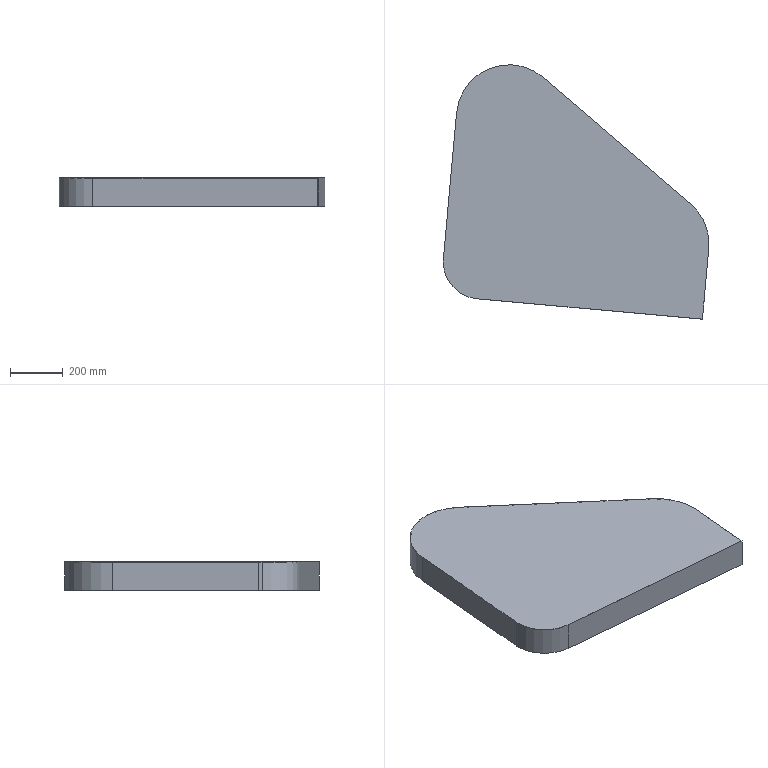Part | SolidWorks | features Extrusion 1, Shell 1 | 1 solid | 19 faces | box 1010 x 967.019 x 110 mm | volume 3119337 mm3 | plane 11 | cylinder 8 | commonest cylinder face diameters 274 x2 280 x2 394 x2 400 x2
STEP:
#1=CARTESIAN_POINT('',(-246.443,-537.657,107.));
#2=VERTEX_POINT('',#1);
#3=CARTESIAN_POINT('',(-247.,-550.,107.));
#4=VERTEX_POINT('',#3);
#5=CARTESIAN_POINT('',(-110.,-550.,107.));
#6=DIRECTION('',(0.,0.,1.));
#7=DIRECTION('',(1.,0.,0.));
#8=AXIS2_PLACEMENT_3D('',#5,#6,#7);
#9=CIRCLE('',#8,137.);
#10=EDGE_CURVE('',#2,#4,#9,.T.);
#11=ORIENTED_EDGE('',*,*,#10,.T.);
#12=CARTESIAN_POINT('',(-247.,-550.,0.));
#13=VERTEX_POINT('',#12);
#14=CARTESIAN_POINT('',(-247.,-550.,110.));
#15=DIRECTION('',(0.,0.,-1.));
#16=VECTOR('',#15,1000.);
#17=LINE('',#14,#16);
#18=EDGE_CURVE('',#4,#13,#17,.T.);
#19=ORIENTED_EDGE('',*,*,#18,.T.);
#20=CARTESIAN_POINT('',(-246.443,-537.657,0.));
#21=VERTEX_POINT('',#20);
#22=CARTESIAN_POINT('',(-110.,-550.,0.));
#23=DIRECTION('',(0.,0.,1.));
#24=DIRECTION('',(1.,0.,0.));
#25=AXIS2_PLACEMENT_3D('',#22,#23,#24);
#26=CIRCLE('',#25,137.);
#27=EDGE_CURVE('',#21,#13,#26,.T.);
#28=ORIENTED_EDGE('',*,*,#27,.F.);
#29=CARTESIAN_POINT('',(-246.443,-537.657,110.));
#30=DIRECTION('',(0.,0.,-1.));
#31=VECTOR('',#30,1000.);
#32=LINE('',#29,#31);
#33=EDGE_CURVE('',#2,#21,#32,.T.);
#34=ORIENTED_EDGE('',*,*,#33,.F.);
#35=EDGE_LOOP('',(#11,#19,#28,#34));
#36=FACE_OUTER_BOUND('',#35,.T.);
#37=CARTESIAN_POINT('',(-110.,-550.,110.));
#38=DIRECTION('',(0.,0.,-1.));
#39=DIRECTION('',(-1.,0.,0.));
#40=AXIS2_PLACEMENT_3D('',#37,#38,#39);
#41=CYLINDRICAL_SURFACE('',#40,137.);
#42=ADVANCED_FACE('',(#36),#41,.F.);
#43=CARTESIAN_POINT('',(-250.,-550.,110.));
#44=VERTEX_POINT('',#43);
#45=CARTESIAN_POINT('',(-122.613,-689.431,110.));
#46=VERTEX_POINT('',#45);
#47=CARTESIAN_POINT('',(-110.,-550.,110.));
#48=DIRECTION('',(0.,0.,1.));
#49=DIRECTION('',(1.,0.,0.));
#50=AXIS2_PLACEMENT_3D('',#47,#48,#49);
#51=CIRCLE('',#50,140.);
#52=EDGE_CURVE('',#44,#46,#51,.T.);
#53=ORIENTED_EDGE('',*,*,#52,.F.);
#54=CARTESIAN_POINT('',(-250.,-550.,0.));
#55=VERTEX_POINT('',#54);
#56=CARTESIAN_POINT('',(-250.,-550.,110.));
#57=DIRECTION('',(0.,0.,-1.));
#58=VECTOR('',#57,1000.);
#59=LINE('',#56,#58);
#60=EDGE_CURVE('',#44,#55,#59,.T.);
#61=ORIENTED_EDGE('',*,*,#60,.T.);
#62=CARTESIAN_POINT('',(-122.613,-689.431,0.));
#63=VERTEX_POINT('',#62);
#64=CARTESIAN_POINT('',(-110.,-550.,0.));
#65=DIRECTION('',(0.,0.,1.));
#66=DIRECTION('',(1.,0.,0.));
#67=AXIS2_PLACEMENT_3D('',#64,#65,#66);
#68=CIRCLE('',#67,140.);
#69=EDGE_CURVE('',#55,#63,#68,.T.);
#70=ORIENTED_EDGE('',*,*,#69,.T.);
#71=CARTESIAN_POINT('',(-122.613,-689.431,110.));
#72=DIRECTION('',(0.,0.,-1.));
#73=VECTOR('',#72,1000.);
#74=LINE('',#71,#73);
#75=EDGE_CURVE('',#46,#63,#74,.T.);
#76=ORIENTED_EDGE('',*,*,#75,.F.);
#77=EDGE_LOOP('',(#53,#61,#70,#76));
#78=FACE_OUTER_BOUND('',#77,.T.);
#79=CARTESIAN_POINT('',(-110.,-550.,110.));
#80=DIRECTION('',(0.,0.,-1.));
#81=DIRECTION('',(-1.,0.,0.));
#82=AXIS2_PLACEMENT_3D('',#79,#80,#81);
#83=CYLINDRICAL_SURFACE('',#82,140.);
#84=ADVANCED_FACE('',(#78),#83,.T.);
#85=CARTESIAN_POINT('',(130.202,151.814,0.));
#86=VERTEX_POINT('',#85);
#87=CARTESIAN_POINT('',(-199.187,18.019,0.));
#88=VERTEX_POINT('',#87);
#89=CARTESIAN_POINT('',(0.,0.,0.));
#90=DIRECTION('',(0.,0.,1.));
#91=DIRECTION('',(1.,0.,0.));
#92=AXIS2_PLACEMENT_3D('',#89,#90,#91);
#93=CIRCLE('',#92,200.);
#94=EDGE_CURVE('',#86,#88,#93,.T.);
#95=ORIENTED_EDGE('',*,*,#94,.T.);
#96=CARTESIAN_POINT('',(-199.187,18.019,110.));
#97=VERTEX_POINT('',#96);
#98=CARTESIAN_POINT('',(-199.187,18.019,110.));
#99=DIRECTION('',(0.,0.,-1.));
#100=VECTOR('',#99,1000.);
#101=LINE('',#98,#100);
#102=EDGE_CURVE('',#97,#88,#101,.T.);
#103=ORIENTED_EDGE('',*,*,#102,.F.);
#104=CARTESIAN_POINT('',(130.202,151.814,110.));
#105=VERTEX_POINT('',#104);
#106=CARTESIAN_POINT('',(0.,0.,110.));
#107=DIRECTION('',(0.,0.,1.));
#108=DIRECTION('',(1.,0.,0.));
#109=AXIS2_PLACEMENT_3D('',#106,#107,#108);
#110=CIRCLE('',#109,200.);
#111=EDGE_CURVE('',#105,#97,#110,.T.);
#112=ORIENTED_EDGE('',*,*,#111,.F.);
#113=CARTESIAN_POINT('',(130.202,151.814,110.));
#114=DIRECTION('',(0.,0.,-1.));
#115=VECTOR('',#114,1000.);
#116=LINE('',#113,#115);
#117=EDGE_CURVE('',#105,#86,#116,.T.);
#118=ORIENTED_EDGE('',*,*,#117,.T.);
#119=EDGE_LOOP('',(#95,#103,#112,#118));
#120=FACE_OUTER_BOUND('',#119,.T.);
#121=CARTESIAN_POINT('',(0.,0.,110.));
#122=DIRECTION('',(0.,0.,-1.));
#123=DIRECTION('',(-1.,0.,0.));
#124=AXIS2_PLACEMENT_3D('',#121,#122,#123);
#125=CYLINDRICAL_SURFACE('',#124,200.);
#126=ADVANCED_FACE('',(#120),#125,.T.);
#127=CARTESIAN_POINT('',(-249.431,-537.387,0.));
#128=VERTEX_POINT('',#127);
#129=CARTESIAN_POINT('',(-199.187,18.019,0.));
#130=DIRECTION('',(-0.0901,-0.9959,0.));
#131=VECTOR('',#130,1000.);
#132=LINE('',#129,#131);
#133=EDGE_CURVE('',#88,#128,#132,.T.);
#134=ORIENTED_EDGE('',*,*,#133,.T.);
#135=CARTESIAN_POINT('',(-249.431,-537.387,110.));
#136=VERTEX_POINT('',#135);
#137=CARTESIAN_POINT('',(-249.431,-537.387,110.));
#138=DIRECTION('',(0.,0.,-1.));
#139=VECTOR('',#138,1000.);
#140=LINE('',#137,#139);
#141=EDGE_CURVE('',#136,#128,#140,.T.);
#142=ORIENTED_EDGE('',*,*,#141,.F.);
#143=CARTESIAN_POINT('',(-199.187,18.019,110.));
#144=DIRECTION('',(-0.0901,-0.9959,0.));
#145=VECTOR('',#144,1000.);
#146=LINE('',#143,#145);
#147=EDGE_CURVE('',#97,#136,#146,.T.);
#148=ORIENTED_EDGE('',*,*,#147,.F.);
#149=ORIENTED_EDGE('',*,*,#102,.T.);
#150=EDGE_LOOP('',(#134,#142,#148,#149));
#151=FACE_OUTER_BOUND('',#150,.T.);
#152=CARTESIAN_POINT('',(-199.187,18.019,110.));
#153=DIRECTION('',(0.9959,-0.0901,0.));
#154=DIRECTION('',(0.0901,0.9959,0.));
#155=AXIS2_PLACEMENT_3D('',#152,#153,#154);
#156=PLANE('',#155);
#157=ADVANCED_FACE('',(#151),#156,.F.);
#158=ORIENTED_EDGE('',*,*,#60,.F.);
#159=CARTESIAN_POINT('',(-110.,-550.,110.));
#160=DIRECTION('',(0.,0.,1.));
#161=DIRECTION('',(1.,0.,0.));
#162=AXIS2_PLACEMENT_3D('',#159,#160,#161);
#163=CIRCLE('',#162,140.);
#164=EDGE_CURVE('',#136,#44,#163,.T.);
#165=ORIENTED_EDGE('',*,*,#164,.F.);
#166=ORIENTED_EDGE('',*,*,#141,.T.);
#167=CARTESIAN_POINT('',(-110.,-550.,0.));
#168=DIRECTION('',(0.,0.,1.));
#169=DIRECTION('',(1.,0.,0.));
#170=AXIS2_PLACEMENT_3D('',#167,#168,#169);
#171=CIRCLE('',#170,140.);
#172=EDGE_CURVE('',#128,#55,#171,.T.);
#173=ORIENTED_EDGE('',*,*,#172,.T.);
#174=EDGE_LOOP('',(#158,#165,#166,#173));
#175=FACE_OUTER_BOUND('',#174,.T.);
#176=CARTESIAN_POINT('',(-110.,-550.,110.));
#177=DIRECTION('',(0.,0.,-1.));
#178=DIRECTION('',(-1.,0.,0.));
#179=AXIS2_PLACEMENT_3D('',#176,#177,#178);
#180=CYLINDRICAL_SURFACE('',#179,140.);
#181=ADVANCED_FACE('',(#175),#180,.T.);
#182=CARTESIAN_POINT('',(735.06,-767.019,0.));
#183=VERTEX_POINT('',#182);
#184=CARTESIAN_POINT('',(-122.613,-689.431,0.));
#185=DIRECTION('',(0.9959,-0.0901,0.));
#186=VECTOR('',#185,1000.);
#187=LINE('',#184,#186);
#188=EDGE_CURVE('',#63,#183,#187,.T.);
#189=ORIENTED_EDGE('',*,*,#188,.T.);
#190=CARTESIAN_POINT('',(735.06,-767.019,110.));
#191=VERTEX_POINT('',#190);
#192=CARTESIAN_POINT('',(735.06,-767.019,110.));
#193=DIRECTION('',(0.,0.,-1.));
#194=VECTOR('',#193,1000.);
#195=LINE('',#192,#194);
#196=EDGE_CURVE('',#191,#183,#195,.T.);
#197=ORIENTED_EDGE('',*,*,#196,.F.);
#198=CARTESIAN_POINT('',(-122.613,-689.431,110.));
#199=DIRECTION('',(0.9959,-0.0901,0.));
#200=VECTOR('',#199,1000.);
#201=LINE('',#198,#200);
#202=EDGE_CURVE('',#46,#191,#201,.T.);
#203=ORIENTED_EDGE('',*,*,#202,.F.);
#204=ORIENTED_EDGE('',*,*,#75,.T.);
#205=EDGE_LOOP('',(#189,#197,#203,#204));
#206=FACE_OUTER_BOUND('',#205,.T.);
#207=CARTESIAN_POINT('',(-122.613,-689.431,110.));
#208=DIRECTION('',(0.0901,0.9959,0.));
#209=DIRECTION('',(-0.9959,0.0901,0.));
#210=AXIS2_PLACEMENT_3D('',#207,#208,#209);
#211=PLANE('',#210);
#212=ADVANCED_FACE('',(#206),#211,.F.);
#213=CARTESIAN_POINT('',(759.356,-498.442,0.));
#214=VERTEX_POINT('',#213);
#215=CARTESIAN_POINT('',(759.356,-498.442,0.));
#216=DIRECTION('',(0.0901,0.9959,0.));
#217=VECTOR('',#216,1000.);
#218=LINE('',#215,#217);
#219=EDGE_CURVE('',#183,#214,#218,.T.);
#220=ORIENTED_EDGE('',*,*,#219,.T.);
#221=CARTESIAN_POINT('',(759.356,-498.442,110.));
#222=VERTEX_POINT('',#221);
#223=CARTESIAN_POINT('',(759.356,-498.442,110.));
#224=DIRECTION('',(0.,0.,-1.));
#225=VECTOR('',#224,1000.);
#226=LINE('',#223,#225);
#227=EDGE_CURVE('',#222,#214,#226,.T.);
#228=ORIENTED_EDGE('',*,*,#227,.F.);
#229=CARTESIAN_POINT('',(759.356,-498.442,110.));
#230=DIRECTION('',(0.0901,0.9959,0.));
#231=VECTOR('',#230,1000.);
#232=LINE('',#229,#231);
#233=EDGE_CURVE('',#191,#222,#232,.T.);
#234=ORIENTED_EDGE('',*,*,#233,.F.);
#235=ORIENTED_EDGE('',*,*,#196,.T.);
#236=EDGE_LOOP('',(#220,#228,#234,#235));
#237=FACE_OUTER_BOUND('',#236,.T.);
#238=CARTESIAN_POINT('',(759.356,-498.442,110.));
#239=DIRECTION('',(-0.9959,0.0901,0.));
#240=DIRECTION('',(-0.0901,-0.9959,0.));
#241=AXIS2_PLACEMENT_3D('',#238,#239,#240);
#242=PLANE('',#241);
#243=ADVANCED_FACE('',(#237),#242,.F.);
#244=CARTESIAN_POINT('',(690.371,-328.609,0.));
#245=VERTEX_POINT('',#244);
#246=CARTESIAN_POINT('',(560.17,-480.423,0.));
#247=DIRECTION('',(0.,0.,1.));
#248=DIRECTION('',(1.,0.,0.));
#249=AXIS2_PLACEMENT_3D('',#246,#247,#248);
#250=CIRCLE('',#249,200.);
#251=EDGE_CURVE('',#214,#245,#250,.T.);
#252=ORIENTED_EDGE('',*,*,#251,.T.);
#253=CARTESIAN_POINT('',(690.371,-328.609,110.));
#254=VERTEX_POINT('',#253);
#255=CARTESIAN_POINT('',(690.371,-328.609,110.));
#256=DIRECTION('',(0.,0.,-1.));
#257=VECTOR('',#256,1000.);
#258=LINE('',#255,#257);
#259=EDGE_CURVE('',#254,#245,#258,.T.);
#260=ORIENTED_EDGE('',*,*,#259,.F.);
#261=CARTESIAN_POINT('',(560.17,-480.423,110.));
#262=DIRECTION('',(0.,0.,1.));
#263=DIRECTION('',(1.,0.,0.));
#264=AXIS2_PLACEMENT_3D('',#261,#262,#263);
#265=CIRCLE('',#264,200.);
#266=EDGE_CURVE('',#222,#254,#265,.T.);
#267=ORIENTED_EDGE('',*,*,#266,.F.);
#268=ORIENTED_EDGE('',*,*,#227,.T.);
#269=EDGE_LOOP('',(#252,#260,#267,#268));
#270=FACE_OUTER_BOUND('',#269,.T.);
#271=CARTESIAN_POINT('',(560.17,-480.423,110.));
#272=DIRECTION('',(0.,0.,-1.));
#273=DIRECTION('',(-1.,0.,0.));
#274=AXIS2_PLACEMENT_3D('',#271,#272,#273);
#275=CYLINDRICAL_SURFACE('',#274,200.);
#276=ADVANCED_FACE('',(#270),#275,.T.);
#277=CARTESIAN_POINT('',(130.202,151.814,0.));
#278=DIRECTION('',(-0.7591,0.651,0.));
#279=VECTOR('',#278,1000.);
#280=LINE('',#277,#279);
#281=EDGE_CURVE('',#245,#86,#280,.T.);
#282=ORIENTED_EDGE('',*,*,#281,.T.);
#283=ORIENTED_EDGE('',*,*,#117,.F.);
#284=CARTESIAN_POINT('',(130.202,151.814,110.));
#285=DIRECTION('',(-0.7591,0.651,0.));
#286=VECTOR('',#285,1000.);
#287=LINE('',#284,#286);
#288=EDGE_CURVE('',#254,#105,#287,.T.);
#289=ORIENTED_EDGE('',*,*,#288,.F.);
#290=ORIENTED_EDGE('',*,*,#259,.T.);
#291=EDGE_LOOP('',(#282,#283,#289,#290));
#292=FACE_OUTER_BOUND('',#291,.T.);
#293=CARTESIAN_POINT('',(130.202,151.814,110.));
#294=DIRECTION('',(-0.651,-0.7591,0.));
#295=DIRECTION('',(0.7591,-0.651,0.));
#296=AXIS2_PLACEMENT_3D('',#293,#294,#295);
#297=PLANE('',#296);
#298=ADVANCED_FACE('',(#292),#297,.F.);
#299=ORIENTED_EDGE('',*,*,#111,.T.);
#300=ORIENTED_EDGE('',*,*,#147,.T.);
#301=ORIENTED_EDGE('',*,*,#164,.T.);
#302=ORIENTED_EDGE('',*,*,#52,.T.);
#303=ORIENTED_EDGE('',*,*,#202,.T.);
#304=ORIENTED_EDGE('',*,*,#233,.T.);
#305=ORIENTED_EDGE('',*,*,#266,.T.);
#306=ORIENTED_EDGE('',*,*,#288,.T.);
#307=EDGE_LOOP('',(#299,#300,#301,#302,#303,#304,#305,#306));
#308=FACE_OUTER_BOUND('',#307,.T.);
#309=CARTESIAN_POINT('',(0.,0.,110.));
#310=DIRECTION('',(0.,0.,1.));
#311=DIRECTION('',(1.,0.,0.));
#312=AXIS2_PLACEMENT_3D('',#309,#310,#311);
#313=PLANE('',#312);
#314=ADVANCED_FACE('',(#308),#313,.T.);
#315=CARTESIAN_POINT('',(688.418,-330.886,0.));
#316=VERTEX_POINT('',#315);
#317=CARTESIAN_POINT('',(128.249,149.537,0.));
#318=VERTEX_POINT('',#317);
#319=CARTESIAN_POINT('',(128.249,149.537,0.));
#320=DIRECTION('',(-0.7591,0.651,0.));
#321=VECTOR('',#320,1000.);
#322=LINE('',#319,#321);
#323=EDGE_CURVE('',#316,#318,#322,.T.);
#324=ORIENTED_EDGE('',*,*,#323,.T.);
#325=CARTESIAN_POINT('',(-196.199,17.749,0.));
#326=VERTEX_POINT('',#325);
#327=CARTESIAN_POINT('',(0.,0.,0.));
#328=DIRECTION('',(0.,0.,1.));
#329=DIRECTION('',(1.,0.,0.));
#330=AXIS2_PLACEMENT_3D('',#327,#328,#329);
#331=CIRCLE('',#330,197.);
#332=EDGE_CURVE('',#318,#326,#331,.T.);
#333=ORIENTED_EDGE('',*,*,#332,.T.);
#334=CARTESIAN_POINT('',(-196.199,17.749,0.));
#335=DIRECTION('',(-0.0901,-0.9959,0.));
#336=VECTOR('',#335,1000.);
#337=LINE('',#334,#336);
#338=EDGE_CURVE('',#326,#21,#337,.T.);
#339=ORIENTED_EDGE('',*,*,#338,.T.);
#340=ORIENTED_EDGE('',*,*,#27,.T.);
#341=CARTESIAN_POINT('',(-122.343,-686.443,0.));
#342=VERTEX_POINT('',#341);
#343=CARTESIAN_POINT('',(-110.,-550.,0.));
#344=DIRECTION('',(0.,0.,1.));
#345=DIRECTION('',(1.,0.,0.));
#346=AXIS2_PLACEMENT_3D('',#343,#344,#345);
#347=CIRCLE('',#346,137.);
#348=EDGE_CURVE('',#13,#342,#347,.T.);
#349=ORIENTED_EDGE('',*,*,#348,.T.);
#350=CARTESIAN_POINT('',(732.342,-763.761,0.));
#351=VERTEX_POINT('',#350);
#352=CARTESIAN_POINT('',(-122.343,-686.443,0.));
#353=DIRECTION('',(0.9959,-0.0901,0.));
#354=VECTOR('',#353,1000.);
#355=LINE('',#352,#354);
#356=EDGE_CURVE('',#342,#351,#355,.T.);
#357=ORIENTED_EDGE('',*,*,#356,.T.);
#358=CARTESIAN_POINT('',(756.368,-498.172,0.));
#359=VERTEX_POINT('',#358);
#360=CARTESIAN_POINT('',(756.368,-498.172,0.));
#361=DIRECTION('',(0.0901,0.9959,0.));
#362=VECTOR('',#361,1000.);
#363=LINE('',#360,#362);
#364=EDGE_CURVE('',#351,#359,#363,.T.);
#365=ORIENTED_EDGE('',*,*,#364,.T.);
#366=CARTESIAN_POINT('',(560.17,-480.423,0.));
#367=DIRECTION('',(0.,0.,1.));
#368=DIRECTION('',(1.,0.,0.));
#369=AXIS2_PLACEMENT_3D('',#366,#367,#368);
#370=CIRCLE('',#369,197.);
#371=EDGE_CURVE('',#359,#316,#370,.T.);
#372=ORIENTED_EDGE('',*,*,#371,.T.);
#373=EDGE_LOOP('',(#324,#333,#339,#340,#349,#357,#365,#372));
#374=FACE_BOUND('',#373,.T.);
#375=ORIENTED_EDGE('',*,*,#94,.F.);
#376=ORIENTED_EDGE('',*,*,#281,.F.);
#377=ORIENTED_EDGE('',*,*,#251,.F.);
#378=ORIENTED_EDGE('',*,*,#219,.F.);
#379=ORIENTED_EDGE('',*,*,#188,.F.);
#380=ORIENTED_EDGE('',*,*,#69,.F.);
#381=ORIENTED_EDGE('',*,*,#172,.F.);
#382=ORIENTED_EDGE('',*,*,#133,.F.);
#383=EDGE_LOOP('',(#375,#376,#377,#378,#379,#380,#381,#382));
#384=FACE_OUTER_BOUND('',#383,.T.);
#385=CARTESIAN_POINT('',(0.,0.,0.));
#386=DIRECTION('',(0.,0.,1.));
#387=DIRECTION('',(1.,0.,0.));
#388=AXIS2_PLACEMENT_3D('',#385,#386,#387);
#389=PLANE('',#388);
#390=ADVANCED_FACE('',(#374,#384),#389,.F.);
#391=ORIENTED_EDGE('',*,*,#332,.F.);
#392=CARTESIAN_POINT('',(128.249,149.537,107.));
#393=VERTEX_POINT('',#392);
#394=CARTESIAN_POINT('',(128.249,149.537,110.));
#395=DIRECTION('',(0.,0.,-1.));
#396=VECTOR('',#395,1000.);
#397=LINE('',#394,#396);
#398=EDGE_CURVE('',#393,#318,#397,.T.);
#399=ORIENTED_EDGE('',*,*,#398,.F.);
#400=CARTESIAN_POINT('',(-196.199,17.749,107.));
#401=VERTEX_POINT('',#400);
#402=CARTESIAN_POINT('',(0.,0.,107.));
#403=DIRECTION('',(0.,0.,1.));
#404=DIRECTION('',(1.,0.,0.));
#405=AXIS2_PLACEMENT_3D('',#402,#403,#404);
#406=CIRCLE('',#405,197.);
#407=EDGE_CURVE('',#393,#401,#406,.T.);
#408=ORIENTED_EDGE('',*,*,#407,.T.);
#409=CARTESIAN_POINT('',(-196.199,17.749,110.));
#410=DIRECTION('',(0.,0.,-1.));
#411=VECTOR('',#410,1000.);
#412=LINE('',#409,#411);
#413=EDGE_CURVE('',#401,#326,#412,.T.);
#414=ORIENTED_EDGE('',*,*,#413,.T.);
#415=EDGE_LOOP('',(#391,#399,#408,#414));
#416=FACE_OUTER_BOUND('',#415,.T.);
#417=CARTESIAN_POINT('',(0.,0.,110.));
#418=DIRECTION('',(0.,0.,-1.));
#419=DIRECTION('',(-1.,0.,0.));
#420=AXIS2_PLACEMENT_3D('',#417,#418,#419);
#421=CYLINDRICAL_SURFACE('',#420,197.);
#422=ADVANCED_FACE('',(#416),#421,.F.);
#423=ORIENTED_EDGE('',*,*,#338,.F.);
#424=ORIENTED_EDGE('',*,*,#413,.F.);
#425=CARTESIAN_POINT('',(-196.199,17.749,107.));
#426=DIRECTION('',(-0.0901,-0.9959,0.));
#427=VECTOR('',#426,1000.);
#428=LINE('',#425,#427);
#429=EDGE_CURVE('',#401,#2,#428,.T.);
#430=ORIENTED_EDGE('',*,*,#429,.T.);
#431=ORIENTED_EDGE('',*,*,#33,.T.);
#432=EDGE_LOOP('',(#423,#424,#430,#431));
#433=FACE_OUTER_BOUND('',#432,.T.);
#434=CARTESIAN_POINT('',(-196.199,17.749,110.));
#435=DIRECTION('',(0.9959,-0.0901,0.));
#436=DIRECTION('',(0.0901,0.9959,0.));
#437=AXIS2_PLACEMENT_3D('',#434,#435,#436);
#438=PLANE('',#437);
#439=ADVANCED_FACE('',(#433),#438,.T.);
#440=ORIENTED_EDGE('',*,*,#18,.F.);
#441=CARTESIAN_POINT('',(-122.343,-686.443,107.));
#442=VERTEX_POINT('',#441);
#443=CARTESIAN_POINT('',(-110.,-550.,107.));
#444=DIRECTION('',(0.,0.,1.));
#445=DIRECTION('',(1.,0.,0.));
#446=AXIS2_PLACEMENT_3D('',#443,#444,#445);
#447=CIRCLE('',#446,137.);
#448=EDGE_CURVE('',#4,#442,#447,.T.);
#449=ORIENTED_EDGE('',*,*,#448,.T.);
#450=CARTESIAN_POINT('',(-122.343,-686.443,110.));
#451=DIRECTION('',(0.,0.,-1.));
#452=VECTOR('',#451,1000.);
#453=LINE('',#450,#452);
#454=EDGE_CURVE('',#442,#342,#453,.T.);
#455=ORIENTED_EDGE('',*,*,#454,.T.);
#456=ORIENTED_EDGE('',*,*,#348,.F.);
#457=EDGE_LOOP('',(#440,#449,#455,#456));
#458=FACE_OUTER_BOUND('',#457,.T.);
#459=CARTESIAN_POINT('',(-110.,-550.,110.));
#460=DIRECTION('',(0.,0.,-1.));
#461=DIRECTION('',(-1.,0.,0.));
#462=AXIS2_PLACEMENT_3D('',#459,#460,#461);
#463=CYLINDRICAL_SURFACE('',#462,137.);
#464=ADVANCED_FACE('',(#458),#463,.F.);
#465=ORIENTED_EDGE('',*,*,#356,.F.);
#466=ORIENTED_EDGE('',*,*,#454,.F.);
#467=CARTESIAN_POINT('',(732.342,-763.761,107.));
#468=VERTEX_POINT('',#467);
#469=CARTESIAN_POINT('',(-122.343,-686.443,107.));
#470=DIRECTION('',(0.9959,-0.0901,0.));
#471=VECTOR('',#470,1000.);
#472=LINE('',#469,#471);
#473=EDGE_CURVE('',#442,#468,#472,.T.);
#474=ORIENTED_EDGE('',*,*,#473,.T.);
#475=CARTESIAN_POINT('',(732.342,-763.761,110.));
#476=DIRECTION('',(0.,0.,-1.));
#477=VECTOR('',#476,1000.);
#478=LINE('',#475,#477);
#479=EDGE_CURVE('',#468,#351,#478,.T.);
#480=ORIENTED_EDGE('',*,*,#479,.T.);
#481=EDGE_LOOP('',(#465,#466,#474,#480));
#482=FACE_OUTER_BOUND('',#481,.T.);
#483=CARTESIAN_POINT('',(-122.343,-686.443,110.));
#484=DIRECTION('',(0.0901,0.9959,0.));
#485=DIRECTION('',(-0.9959,0.0901,0.));
#486=AXIS2_PLACEMENT_3D('',#483,#484,#485);
#487=PLANE('',#486);
#488=ADVANCED_FACE('',(#482),#487,.T.);
#489=ORIENTED_EDGE('',*,*,#364,.F.);
#490=ORIENTED_EDGE('',*,*,#479,.F.);
#491=CARTESIAN_POINT('',(756.368,-498.172,107.));
#492=VERTEX_POINT('',#491);
#493=CARTESIAN_POINT('',(756.368,-498.172,107.));
#494=DIRECTION('',(0.0901,0.9959,0.));
#495=VECTOR('',#494,1000.);
#496=LINE('',#493,#495);
#497=EDGE_CURVE('',#468,#492,#496,.T.);
#498=ORIENTED_EDGE('',*,*,#497,.T.);
#499=CARTESIAN_POINT('',(756.368,-498.172,110.));
#500=DIRECTION('',(0.,0.,-1.));
#501=VECTOR('',#500,1000.);
#502=LINE('',#499,#501);
#503=EDGE_CURVE('',#492,#359,#502,.T.);
#504=ORIENTED_EDGE('',*,*,#503,.T.);
#505=EDGE_LOOP('',(#489,#490,#498,#504));
#506=FACE_OUTER_BOUND('',#505,.T.);
#507=CARTESIAN_POINT('',(756.368,-498.172,110.));
#508=DIRECTION('',(-0.9959,0.0901,0.));
#509=DIRECTION('',(-0.0901,-0.9959,0.));
#510=AXIS2_PLACEMENT_3D('',#507,#508,#509);
#511=PLANE('',#510);
#512=ADVANCED_FACE('',(#506),#511,.T.);
#513=ORIENTED_EDGE('',*,*,#371,.F.);
#514=ORIENTED_EDGE('',*,*,#503,.F.);
#515=CARTESIAN_POINT('',(688.418,-330.886,107.));
#516=VERTEX_POINT('',#515);
#517=CARTESIAN_POINT('',(560.17,-480.423,107.));
#518=DIRECTION('',(0.,0.,1.));
#519=DIRECTION('',(1.,0.,0.));
#520=AXIS2_PLACEMENT_3D('',#517,#518,#519);
#521=CIRCLE('',#520,197.);
#522=EDGE_CURVE('',#492,#516,#521,.T.);
#523=ORIENTED_EDGE('',*,*,#522,.T.);
#524=CARTESIAN_POINT('',(688.418,-330.886,110.));
#525=DIRECTION('',(0.,0.,-1.));
#526=VECTOR('',#525,1000.);
#527=LINE('',#524,#526);
#528=EDGE_CURVE('',#516,#316,#527,.T.);
#529=ORIENTED_EDGE('',*,*,#528,.T.);
#530=EDGE_LOOP('',(#513,#514,#523,#529));
#531=FACE_OUTER_BOUND('',#530,.T.);
#532=CARTESIAN_POINT('',(560.17,-480.423,110.));
#533=DIRECTION('',(0.,0.,-1.));
#534=DIRECTION('',(-1.,0.,0.));
#535=AXIS2_PLACEMENT_3D('',#532,#533,#534);
#536=CYLINDRICAL_SURFACE('',#535,197.);
#537=ADVANCED_FACE('',(#531),#536,.F.);
#538=ORIENTED_EDGE('',*,*,#323,.F.);
#539=ORIENTED_EDGE('',*,*,#528,.F.);
#540=CARTESIAN_POINT('',(128.249,149.537,107.));
#541=DIRECTION('',(-0.7591,0.651,0.));
#542=VECTOR('',#541,1000.);
#543=LINE('',#540,#542);
#544=EDGE_CURVE('',#516,#393,#543,.T.);
#545=ORIENTED_EDGE('',*,*,#544,.T.);
#546=ORIENTED_EDGE('',*,*,#398,.T.);
#547=EDGE_LOOP('',(#538,#539,#545,#546));
#548=FACE_OUTER_BOUND('',#547,.T.);
#549=CARTESIAN_POINT('',(128.249,149.537,110.));
#550=DIRECTION('',(-0.651,-0.7591,0.));
#551=DIRECTION('',(0.7591,-0.651,0.));
#552=AXIS2_PLACEMENT_3D('',#549,#550,#551);
#553=PLANE('',#552);
#554=ADVANCED_FACE('',(#548),#553,.T.);
#555=ORIENTED_EDGE('',*,*,#407,.F.);
#556=ORIENTED_EDGE('',*,*,#544,.F.);
#557=ORIENTED_EDGE('',*,*,#522,.F.);
#558=ORIENTED_EDGE('',*,*,#497,.F.);
#559=ORIENTED_EDGE('',*,*,#473,.F.);
#560=ORIENTED_EDGE('',*,*,#448,.F.);
#561=ORIENTED_EDGE('',*,*,#10,.F.);
#562=ORIENTED_EDGE('',*,*,#429,.F.);
#563=EDGE_LOOP('',(#555,#556,#557,#558,#559,#560,#561,#562));
#564=FACE_OUTER_BOUND('',#563,.T.);
#565=CARTESIAN_POINT('',(0.,0.,107.));
#566=DIRECTION('',(0.,0.,1.));
#567=DIRECTION('',(1.,0.,0.));
#568=AXIS2_PLACEMENT_3D('',#565,#566,#567);
#569=PLANE('',#568);
#570=ADVANCED_FACE('',(#564),#569,.F.);
#571=CLOSED_SHELL('',(#42,#84,#126,#157,#181,#212,#243,#276,#298,#314,#390,#422,#439,#464,#488,#512,#537,#554,#570));
#572=MANIFOLD_SOLID_BREP('',#571);
#573=CARTESIAN_POINT('',(0.,0.,0.));
#574=DIRECTION('',(0.,0.,1.));
#575=DIRECTION('',(1.,0.,0.));
#576=AXIS2_PLACEMENT_3D('',#573,#574,#575);
#577=(LENGTH_UNIT()NAMED_UNIT(*)SI_UNIT(.MILLI.,.METRE.));
#578=UNCERTAINTY_MEASURE_WITH_UNIT(LENGTH_MEASURE(0.00001),#577,'','');
#579=(NAMED_UNIT(*)PLANE_ANGLE_UNIT()SI_UNIT($,.RADIAN.));
#580=(NAMED_UNIT(*)SI_UNIT($,.STERADIAN.)SOLID_ANGLE_UNIT());
#581=(GEOMETRIC_REPRESENTATION_CONTEXT(3)GLOBAL_UNCERTAINTY_ASSIGNED_CONTEXT((#578))GLOBAL_UNIT_ASSIGNED_CONTEXT((#577,#579,#580))REPRESENTATION_CONTEXT('',''));
#582=ADVANCED_BREP_SHAPE_REPRESENTATION('',(#572,#576),#581);